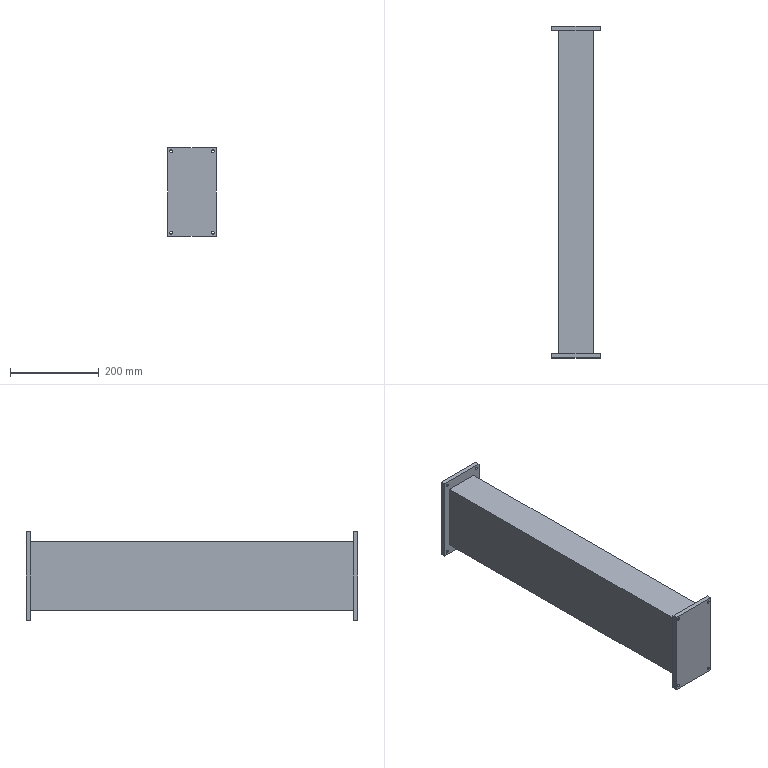Part | SolidWorks | features ICE 2, Extrusion 1 | 1 solid | 32 faces | box 110 x 750 x 200 mm | volume 9118663 mm3 | cylinder 16 | plane 16 | commonest cylinder face diameters 6.5 x16
STEP:
#1=CARTESIAN_POINT('',(-47.,750.,88.75));
#2=VERTEX_POINT('',#1);
#3=CARTESIAN_POINT('',(-47.,750.,95.25));
#4=VERTEX_POINT('',#3);
#5=CARTESIAN_POINT('',(-47.,750.,92.));
#6=DIRECTION('',(0.,1.,0.));
#7=DIRECTION('',(0.,0.,1.));
#8=AXIS2_PLACEMENT_3D('',#5,#6,#7);
#9=CIRCLE('',#8,3.25);
#10=EDGE_CURVE('',#2,#4,#9,.T.);
#11=ORIENTED_EDGE('',*,*,#10,.T.);
#12=CARTESIAN_POINT('',(-47.,740.,95.25));
#13=VERTEX_POINT('',#12);
#14=CARTESIAN_POINT('',(-47.,750.,95.25));
#15=DIRECTION('',(0.,-1.,0.));
#16=VECTOR('',#15,1000.);
#17=LINE('',#14,#16);
#18=EDGE_CURVE('',#4,#13,#17,.T.);
#19=ORIENTED_EDGE('',*,*,#18,.T.);
#20=CARTESIAN_POINT('',(-47.,740.,88.75));
#21=VERTEX_POINT('',#20);
#22=CARTESIAN_POINT('',(-47.,740.,92.));
#23=DIRECTION('',(0.,1.,0.));
#24=DIRECTION('',(0.,0.,1.));
#25=AXIS2_PLACEMENT_3D('',#22,#23,#24);
#26=CIRCLE('',#25,3.25);
#27=EDGE_CURVE('',#21,#13,#26,.T.);
#28=ORIENTED_EDGE('',*,*,#27,.F.);
#29=CARTESIAN_POINT('',(-47.,750.,88.75));
#30=DIRECTION('',(0.,-1.,0.));
#31=VECTOR('',#30,1000.);
#32=LINE('',#29,#31);
#33=EDGE_CURVE('',#2,#21,#32,.T.);
#34=ORIENTED_EDGE('',*,*,#33,.F.);
#35=EDGE_LOOP('',(#11,#19,#28,#34));
#36=FACE_OUTER_BOUND('',#35,.T.);
#37=CARTESIAN_POINT('',(-47.,750.,92.));
#38=DIRECTION('',(0.,-1.,0.));
#39=DIRECTION('',(0.,0.,-1.));
#40=AXIS2_PLACEMENT_3D('',#37,#38,#39);
#41=CYLINDRICAL_SURFACE('',#40,3.25);
#42=ADVANCED_FACE('',(#36),#41,.F.);
#43=CARTESIAN_POINT('',(47.,750.,88.75));
#44=VERTEX_POINT('',#43);
#45=CARTESIAN_POINT('',(47.,750.,95.25));
#46=VERTEX_POINT('',#45);
#47=CARTESIAN_POINT('',(47.,750.,92.));
#48=DIRECTION('',(0.,1.,0.));
#49=DIRECTION('',(0.,0.,1.));
#50=AXIS2_PLACEMENT_3D('',#47,#48,#49);
#51=CIRCLE('',#50,3.25);
#52=EDGE_CURVE('',#44,#46,#51,.T.);
#53=ORIENTED_EDGE('',*,*,#52,.T.);
#54=CARTESIAN_POINT('',(47.,740.,95.25));
#55=VERTEX_POINT('',#54);
#56=CARTESIAN_POINT('',(47.,750.,95.25));
#57=DIRECTION('',(0.,-1.,0.));
#58=VECTOR('',#57,1000.);
#59=LINE('',#56,#58);
#60=EDGE_CURVE('',#46,#55,#59,.T.);
#61=ORIENTED_EDGE('',*,*,#60,.T.);
#62=CARTESIAN_POINT('',(47.,740.,88.75));
#63=VERTEX_POINT('',#62);
#64=CARTESIAN_POINT('',(47.,740.,92.));
#65=DIRECTION('',(0.,1.,0.));
#66=DIRECTION('',(0.,0.,1.));
#67=AXIS2_PLACEMENT_3D('',#64,#65,#66);
#68=CIRCLE('',#67,3.25);
#69=EDGE_CURVE('',#63,#55,#68,.T.);
#70=ORIENTED_EDGE('',*,*,#69,.F.);
#71=CARTESIAN_POINT('',(47.,750.,88.75));
#72=DIRECTION('',(0.,-1.,0.));
#73=VECTOR('',#72,1000.);
#74=LINE('',#71,#73);
#75=EDGE_CURVE('',#44,#63,#74,.T.);
#76=ORIENTED_EDGE('',*,*,#75,.F.);
#77=EDGE_LOOP('',(#53,#61,#70,#76));
#78=FACE_OUTER_BOUND('',#77,.T.);
#79=CARTESIAN_POINT('',(47.,750.,92.));
#80=DIRECTION('',(0.,-1.,0.));
#81=DIRECTION('',(0.,0.,-1.));
#82=AXIS2_PLACEMENT_3D('',#79,#80,#81);
#83=CYLINDRICAL_SURFACE('',#82,3.25);
#84=ADVANCED_FACE('',(#78),#83,.F.);
#85=CARTESIAN_POINT('',(47.,750.,-95.25));
#86=VERTEX_POINT('',#85);
#87=CARTESIAN_POINT('',(47.,750.,-88.75));
#88=VERTEX_POINT('',#87);
#89=CARTESIAN_POINT('',(47.,750.,-92.));
#90=DIRECTION('',(0.,1.,0.));
#91=DIRECTION('',(0.,0.,1.));
#92=AXIS2_PLACEMENT_3D('',#89,#90,#91);
#93=CIRCLE('',#92,3.25);
#94=EDGE_CURVE('',#86,#88,#93,.T.);
#95=ORIENTED_EDGE('',*,*,#94,.T.);
#96=CARTESIAN_POINT('',(47.,740.,-88.75));
#97=VERTEX_POINT('',#96);
#98=CARTESIAN_POINT('',(47.,750.,-88.75));
#99=DIRECTION('',(0.,-1.,0.));
#100=VECTOR('',#99,1000.);
#101=LINE('',#98,#100);
#102=EDGE_CURVE('',#88,#97,#101,.T.);
#103=ORIENTED_EDGE('',*,*,#102,.T.);
#104=CARTESIAN_POINT('',(47.,740.,-95.25));
#105=VERTEX_POINT('',#104);
#106=CARTESIAN_POINT('',(47.,740.,-92.));
#107=DIRECTION('',(0.,1.,0.));
#108=DIRECTION('',(0.,0.,1.));
#109=AXIS2_PLACEMENT_3D('',#106,#107,#108);
#110=CIRCLE('',#109,3.25);
#111=EDGE_CURVE('',#105,#97,#110,.T.);
#112=ORIENTED_EDGE('',*,*,#111,.F.);
#113=CARTESIAN_POINT('',(47.,750.,-95.25));
#114=DIRECTION('',(0.,-1.,0.));
#115=VECTOR('',#114,1000.);
#116=LINE('',#113,#115);
#117=EDGE_CURVE('',#86,#105,#116,.T.);
#118=ORIENTED_EDGE('',*,*,#117,.F.);
#119=EDGE_LOOP('',(#95,#103,#112,#118));
#120=FACE_OUTER_BOUND('',#119,.T.);
#121=CARTESIAN_POINT('',(47.,750.,-92.));
#122=DIRECTION('',(0.,-1.,0.));
#123=DIRECTION('',(0.,0.,-1.));
#124=AXIS2_PLACEMENT_3D('',#121,#122,#123);
#125=CYLINDRICAL_SURFACE('',#124,3.25);
#126=ADVANCED_FACE('',(#120),#125,.F.);
#127=CARTESIAN_POINT('',(-47.,750.,-95.25));
#128=VERTEX_POINT('',#127);
#129=CARTESIAN_POINT('',(-47.,750.,-88.75));
#130=VERTEX_POINT('',#129);
#131=CARTESIAN_POINT('',(-47.,750.,-92.));
#132=DIRECTION('',(0.,1.,0.));
#133=DIRECTION('',(0.,0.,1.));
#134=AXIS2_PLACEMENT_3D('',#131,#132,#133);
#135=CIRCLE('',#134,3.25);
#136=EDGE_CURVE('',#128,#130,#135,.T.);
#137=ORIENTED_EDGE('',*,*,#136,.T.);
#138=CARTESIAN_POINT('',(-47.,740.,-88.75));
#139=VERTEX_POINT('',#138);
#140=CARTESIAN_POINT('',(-47.,750.,-88.75));
#141=DIRECTION('',(0.,-1.,0.));
#142=VECTOR('',#141,1000.);
#143=LINE('',#140,#142);
#144=EDGE_CURVE('',#130,#139,#143,.T.);
#145=ORIENTED_EDGE('',*,*,#144,.T.);
#146=CARTESIAN_POINT('',(-47.,740.,-95.25));
#147=VERTEX_POINT('',#146);
#148=CARTESIAN_POINT('',(-47.,740.,-92.));
#149=DIRECTION('',(0.,1.,0.));
#150=DIRECTION('',(0.,0.,1.));
#151=AXIS2_PLACEMENT_3D('',#148,#149,#150);
#152=CIRCLE('',#151,3.25);
#153=EDGE_CURVE('',#147,#139,#152,.T.);
#154=ORIENTED_EDGE('',*,*,#153,.F.);
#155=CARTESIAN_POINT('',(-47.,750.,-95.25));
#156=DIRECTION('',(0.,-1.,0.));
#157=VECTOR('',#156,1000.);
#158=LINE('',#155,#157);
#159=EDGE_CURVE('',#128,#147,#158,.T.);
#160=ORIENTED_EDGE('',*,*,#159,.F.);
#161=EDGE_LOOP('',(#137,#145,#154,#160));
#162=FACE_OUTER_BOUND('',#161,.T.);
#163=CARTESIAN_POINT('',(-47.,750.,-92.));
#164=DIRECTION('',(0.,-1.,0.));
#165=DIRECTION('',(0.,0.,-1.));
#166=AXIS2_PLACEMENT_3D('',#163,#164,#165);
#167=CYLINDRICAL_SURFACE('',#166,3.25);
#168=ADVANCED_FACE('',(#162),#167,.F.);
#169=CARTESIAN_POINT('',(-47.,10.,88.75));
#170=VERTEX_POINT('',#169);
#171=CARTESIAN_POINT('',(-47.,10.,95.25));
#172=VERTEX_POINT('',#171);
#173=CARTESIAN_POINT('',(-47.,10.,92.));
#174=DIRECTION('',(0.,1.,0.));
#175=DIRECTION('',(0.,0.,1.));
#176=AXIS2_PLACEMENT_3D('',#173,#174,#175);
#177=CIRCLE('',#176,3.25);
#178=EDGE_CURVE('',#170,#172,#177,.T.);
#179=ORIENTED_EDGE('',*,*,#178,.T.);
#180=CARTESIAN_POINT('',(-47.,0.,95.25));
#181=VERTEX_POINT('',#180);
#182=CARTESIAN_POINT('',(-47.,10.,95.25));
#183=DIRECTION('',(0.,-1.,0.));
#184=VECTOR('',#183,1000.);
#185=LINE('',#182,#184);
#186=EDGE_CURVE('',#172,#181,#185,.T.);
#187=ORIENTED_EDGE('',*,*,#186,.T.);
#188=CARTESIAN_POINT('',(-47.,0.,88.75));
#189=VERTEX_POINT('',#188);
#190=CARTESIAN_POINT('',(-47.,0.,92.));
#191=DIRECTION('',(0.,1.,0.));
#192=DIRECTION('',(0.,0.,1.));
#193=AXIS2_PLACEMENT_3D('',#190,#191,#192);
#194=CIRCLE('',#193,3.25);
#195=EDGE_CURVE('',#189,#181,#194,.T.);
#196=ORIENTED_EDGE('',*,*,#195,.F.);
#197=CARTESIAN_POINT('',(-47.,10.,88.75));
#198=DIRECTION('',(0.,-1.,0.));
#199=VECTOR('',#198,1000.);
#200=LINE('',#197,#199);
#201=EDGE_CURVE('',#170,#189,#200,.T.);
#202=ORIENTED_EDGE('',*,*,#201,.F.);
#203=EDGE_LOOP('',(#179,#187,#196,#202));
#204=FACE_OUTER_BOUND('',#203,.T.);
#205=CARTESIAN_POINT('',(-47.,10.,92.));
#206=DIRECTION('',(0.,-1.,0.));
#207=DIRECTION('',(0.,0.,-1.));
#208=AXIS2_PLACEMENT_3D('',#205,#206,#207);
#209=CYLINDRICAL_SURFACE('',#208,3.25);
#210=ADVANCED_FACE('',(#204),#209,.F.);
#211=CARTESIAN_POINT('',(47.,10.,88.75));
#212=VERTEX_POINT('',#211);
#213=CARTESIAN_POINT('',(47.,10.,95.25));
#214=VERTEX_POINT('',#213);
#215=CARTESIAN_POINT('',(47.,10.,92.));
#216=DIRECTION('',(0.,1.,0.));
#217=DIRECTION('',(0.,0.,1.));
#218=AXIS2_PLACEMENT_3D('',#215,#216,#217);
#219=CIRCLE('',#218,3.25);
#220=EDGE_CURVE('',#212,#214,#219,.T.);
#221=ORIENTED_EDGE('',*,*,#220,.T.);
#222=CARTESIAN_POINT('',(47.,0.,95.25));
#223=VERTEX_POINT('',#222);
#224=CARTESIAN_POINT('',(47.,10.,95.25));
#225=DIRECTION('',(0.,-1.,0.));
#226=VECTOR('',#225,1000.);
#227=LINE('',#224,#226);
#228=EDGE_CURVE('',#214,#223,#227,.T.);
#229=ORIENTED_EDGE('',*,*,#228,.T.);
#230=CARTESIAN_POINT('',(47.,0.,88.75));
#231=VERTEX_POINT('',#230);
#232=CARTESIAN_POINT('',(47.,0.,92.));
#233=DIRECTION('',(0.,1.,0.));
#234=DIRECTION('',(0.,0.,1.));
#235=AXIS2_PLACEMENT_3D('',#232,#233,#234);
#236=CIRCLE('',#235,3.25);
#237=EDGE_CURVE('',#231,#223,#236,.T.);
#238=ORIENTED_EDGE('',*,*,#237,.F.);
#239=CARTESIAN_POINT('',(47.,10.,88.75));
#240=DIRECTION('',(0.,-1.,0.));
#241=VECTOR('',#240,1000.);
#242=LINE('',#239,#241);
#243=EDGE_CURVE('',#212,#231,#242,.T.);
#244=ORIENTED_EDGE('',*,*,#243,.F.);
#245=EDGE_LOOP('',(#221,#229,#238,#244));
#246=FACE_OUTER_BOUND('',#245,.T.);
#247=CARTESIAN_POINT('',(47.,10.,92.));
#248=DIRECTION('',(0.,-1.,0.));
#249=DIRECTION('',(0.,0.,-1.));
#250=AXIS2_PLACEMENT_3D('',#247,#248,#249);
#251=CYLINDRICAL_SURFACE('',#250,3.25);
#252=ADVANCED_FACE('',(#246),#251,.F.);
#253=CARTESIAN_POINT('',(47.,10.,-95.25));
#254=VERTEX_POINT('',#253);
#255=CARTESIAN_POINT('',(47.,10.,-88.75));
#256=VERTEX_POINT('',#255);
#257=CARTESIAN_POINT('',(47.,10.,-92.));
#258=DIRECTION('',(0.,1.,0.));
#259=DIRECTION('',(0.,0.,1.));
#260=AXIS2_PLACEMENT_3D('',#257,#258,#259);
#261=CIRCLE('',#260,3.25);
#262=EDGE_CURVE('',#254,#256,#261,.T.);
#263=ORIENTED_EDGE('',*,*,#262,.T.);
#264=CARTESIAN_POINT('',(47.,0.,-88.75));
#265=VERTEX_POINT('',#264);
#266=CARTESIAN_POINT('',(47.,10.,-88.75));
#267=DIRECTION('',(0.,-1.,0.));
#268=VECTOR('',#267,1000.);
#269=LINE('',#266,#268);
#270=EDGE_CURVE('',#256,#265,#269,.T.);
#271=ORIENTED_EDGE('',*,*,#270,.T.);
#272=CARTESIAN_POINT('',(47.,0.,-95.25));
#273=VERTEX_POINT('',#272);
#274=CARTESIAN_POINT('',(47.,0.,-92.));
#275=DIRECTION('',(0.,1.,0.));
#276=DIRECTION('',(0.,0.,1.));
#277=AXIS2_PLACEMENT_3D('',#274,#275,#276);
#278=CIRCLE('',#277,3.25);
#279=EDGE_CURVE('',#273,#265,#278,.T.);
#280=ORIENTED_EDGE('',*,*,#279,.F.);
#281=CARTESIAN_POINT('',(47.,10.,-95.25));
#282=DIRECTION('',(0.,-1.,0.));
#283=VECTOR('',#282,1000.);
#284=LINE('',#281,#283);
#285=EDGE_CURVE('',#254,#273,#284,.T.);
#286=ORIENTED_EDGE('',*,*,#285,.F.);
#287=EDGE_LOOP('',(#263,#271,#280,#286));
#288=FACE_OUTER_BOUND('',#287,.T.);
#289=CARTESIAN_POINT('',(47.,10.,-92.));
#290=DIRECTION('',(0.,-1.,0.));
#291=DIRECTION('',(0.,0.,-1.));
#292=AXIS2_PLACEMENT_3D('',#289,#290,#291);
#293=CYLINDRICAL_SURFACE('',#292,3.25);
#294=ADVANCED_FACE('',(#288),#293,.F.);
#295=CARTESIAN_POINT('',(-47.,10.,-95.25));
#296=VERTEX_POINT('',#295);
#297=CARTESIAN_POINT('',(-47.,10.,-88.75));
#298=VERTEX_POINT('',#297);
#299=CARTESIAN_POINT('',(-47.,10.,-92.));
#300=DIRECTION('',(0.,1.,0.));
#301=DIRECTION('',(0.,0.,1.));
#302=AXIS2_PLACEMENT_3D('',#299,#300,#301);
#303=CIRCLE('',#302,3.25);
#304=EDGE_CURVE('',#296,#298,#303,.T.);
#305=ORIENTED_EDGE('',*,*,#304,.T.);
#306=CARTESIAN_POINT('',(-47.,0.,-88.75));
#307=VERTEX_POINT('',#306);
#308=CARTESIAN_POINT('',(-47.,10.,-88.75));
#309=DIRECTION('',(0.,-1.,0.));
#310=VECTOR('',#309,1000.);
#311=LINE('',#308,#310);
#312=EDGE_CURVE('',#298,#307,#311,.T.);
#313=ORIENTED_EDGE('',*,*,#312,.T.);
#314=CARTESIAN_POINT('',(-47.,0.,-95.25));
#315=VERTEX_POINT('',#314);
#316=CARTESIAN_POINT('',(-47.,0.,-92.));
#317=DIRECTION('',(0.,1.,0.));
#318=DIRECTION('',(0.,0.,1.));
#319=AXIS2_PLACEMENT_3D('',#316,#317,#318);
#320=CIRCLE('',#319,3.25);
#321=EDGE_CURVE('',#315,#307,#320,.T.);
#322=ORIENTED_EDGE('',*,*,#321,.F.);
#323=CARTESIAN_POINT('',(-47.,10.,-95.25));
#324=DIRECTION('',(0.,-1.,0.));
#325=VECTOR('',#324,1000.);
#326=LINE('',#323,#325);
#327=EDGE_CURVE('',#296,#315,#326,.T.);
#328=ORIENTED_EDGE('',*,*,#327,.F.);
#329=EDGE_LOOP('',(#305,#313,#322,#328));
#330=FACE_OUTER_BOUND('',#329,.T.);
#331=CARTESIAN_POINT('',(-47.,10.,-92.));
#332=DIRECTION('',(0.,-1.,0.));
#333=DIRECTION('',(0.,0.,-1.));
#334=AXIS2_PLACEMENT_3D('',#331,#332,#333);
#335=CYLINDRICAL_SURFACE('',#334,3.25);
#336=ADVANCED_FACE('',(#330),#335,.F.);
#337=ORIENTED_EDGE('',*,*,#178,.F.);
#338=CARTESIAN_POINT('',(-47.,10.,92.));
#339=DIRECTION('',(0.,1.,0.));
#340=DIRECTION('',(0.,0.,1.));
#341=AXIS2_PLACEMENT_3D('',#338,#339,#340);
#342=CIRCLE('',#341,3.25);
#343=EDGE_CURVE('',#172,#170,#342,.T.);
#344=ORIENTED_EDGE('',*,*,#343,.F.);
#345=EDGE_LOOP('',(#337,#344));
#346=FACE_BOUND('',#345,.T.);
#347=ORIENTED_EDGE('',*,*,#220,.F.);
#348=CARTESIAN_POINT('',(47.,10.,92.));
#349=DIRECTION('',(0.,1.,0.));
#350=DIRECTION('',(0.,0.,1.));
#351=AXIS2_PLACEMENT_3D('',#348,#349,#350);
#352=CIRCLE('',#351,3.25);
#353=EDGE_CURVE('',#214,#212,#352,.T.);
#354=ORIENTED_EDGE('',*,*,#353,.F.);
#355=EDGE_LOOP('',(#347,#354));
#356=FACE_BOUND('',#355,.T.);
#357=ORIENTED_EDGE('',*,*,#262,.F.);
#358=CARTESIAN_POINT('',(47.,10.,-92.));
#359=DIRECTION('',(0.,1.,0.));
#360=DIRECTION('',(0.,0.,1.));
#361=AXIS2_PLACEMENT_3D('',#358,#359,#360);
#362=CIRCLE('',#361,3.25);
#363=EDGE_CURVE('',#256,#254,#362,.T.);
#364=ORIENTED_EDGE('',*,*,#363,.F.);
#365=EDGE_LOOP('',(#357,#364));
#366=FACE_BOUND('',#365,.T.);
#367=ORIENTED_EDGE('',*,*,#304,.F.);
#368=CARTESIAN_POINT('',(-47.,10.,-92.));
#369=DIRECTION('',(0.,1.,0.));
#370=DIRECTION('',(0.,0.,1.));
#371=AXIS2_PLACEMENT_3D('',#368,#369,#370);
#372=CIRCLE('',#371,3.25);
#373=EDGE_CURVE('',#298,#296,#372,.T.);
#374=ORIENTED_EDGE('',*,*,#373,.F.);
#375=EDGE_LOOP('',(#367,#374));
#376=FACE_BOUND('',#375,.T.);
#377=CARTESIAN_POINT('',(55.,10.,100.));
#378=VERTEX_POINT('',#377);
#379=CARTESIAN_POINT('',(55.,10.,-100.));
#380=VERTEX_POINT('',#379);
#381=CARTESIAN_POINT('',(55.,10.,100.));
#382=DIRECTION('',(0.,0.,-1.));
#383=VECTOR('',#382,1000.);
#384=LINE('',#381,#383);
#385=EDGE_CURVE('',#378,#380,#384,.T.);
#386=ORIENTED_EDGE('',*,*,#385,.T.);
#387=CARTESIAN_POINT('',(-55.,10.,-100.));
#388=VERTEX_POINT('',#387);
#389=CARTESIAN_POINT('',(-55.,10.,-100.));
#390=DIRECTION('',(-1.,0.,0.));
#391=VECTOR('',#390,1000.);
#392=LINE('',#389,#391);
#393=EDGE_CURVE('',#380,#388,#392,.T.);
#394=ORIENTED_EDGE('',*,*,#393,.T.);
#395=CARTESIAN_POINT('',(-55.,10.,100.));
#396=VERTEX_POINT('',#395);
#397=CARTESIAN_POINT('',(-55.,10.,100.));
#398=DIRECTION('',(0.,0.,1.));
#399=VECTOR('',#398,1000.);
#400=LINE('',#397,#399);
#401=EDGE_CURVE('',#388,#396,#400,.T.);
#402=ORIENTED_EDGE('',*,*,#401,.T.);
#403=CARTESIAN_POINT('',(-55.,10.,100.));
#404=DIRECTION('',(1.,0.,0.));
#405=VECTOR('',#404,1000.);
#406=LINE('',#403,#405);
#407=EDGE_CURVE('',#396,#378,#406,.T.);
#408=ORIENTED_EDGE('',*,*,#407,.T.);
#409=EDGE_LOOP('',(#386,#394,#402,#408));
#410=FACE_OUTER_BOUND('',#409,.T.);
#411=CARTESIAN_POINT('',(38.672,10.,76.878));
#412=VERTEX_POINT('',#411);
#413=CARTESIAN_POINT('',(38.672,10.,-76.878));
#414=VERTEX_POINT('',#413);
#415=CARTESIAN_POINT('',(38.672,10.,76.878));
#416=DIRECTION('',(0.,0.,-1.));
#417=VECTOR('',#416,1000.);
#418=LINE('',#415,#417);
#419=EDGE_CURVE('',#412,#414,#418,.T.);
#420=ORIENTED_EDGE('',*,*,#419,.F.);
#421=CARTESIAN_POINT('',(-38.672,10.,76.878));
#422=VERTEX_POINT('',#421);
#423=CARTESIAN_POINT('',(-38.672,10.,76.878));
#424=DIRECTION('',(1.,0.,0.));
#425=VECTOR('',#424,1000.);
#426=LINE('',#423,#425);
#427=EDGE_CURVE('',#422,#412,#426,.T.);
#428=ORIENTED_EDGE('',*,*,#427,.F.);
#429=CARTESIAN_POINT('',(-38.672,10.,-76.878));
#430=VERTEX_POINT('',#429);
#431=CARTESIAN_POINT('',(-38.672,10.,76.878));
#432=DIRECTION('',(0.,0.,1.));
#433=VECTOR('',#432,1000.);
#434=LINE('',#431,#433);
#435=EDGE_CURVE('',#430,#422,#434,.T.);
#436=ORIENTED_EDGE('',*,*,#435,.F.);
#437=CARTESIAN_POINT('',(-38.672,10.,-76.878));
#438=DIRECTION('',(-1.,0.,0.));
#439=VECTOR('',#438,1000.);
#440=LINE('',#437,#439);
#441=EDGE_CURVE('',#414,#430,#440,.T.);
#442=ORIENTED_EDGE('',*,*,#441,.F.);
#443=EDGE_LOOP('',(#420,#428,#436,#442));
#444=FACE_BOUND('',#443,.T.);
#445=CARTESIAN_POINT('',(0.,10.,0.));
#446=DIRECTION('',(0.,-1.,0.));
#447=DIRECTION('',(0.,0.,-1.));
#448=AXIS2_PLACEMENT_3D('',#445,#446,#447);
#449=PLANE('',#448);
#450=ADVANCED_FACE('',(#346,#356,#366,#376,#410,#444),#449,.F.);
#451=ORIENTED_EDGE('',*,*,#237,.T.);
#452=CARTESIAN_POINT('',(47.,0.,92.));
#453=DIRECTION('',(0.,1.,0.));
#454=DIRECTION('',(0.,0.,1.));
#455=AXIS2_PLACEMENT_3D('',#452,#453,#454);
#456=CIRCLE('',#455,3.25);
#457=EDGE_CURVE('',#223,#231,#456,.T.);
#458=ORIENTED_EDGE('',*,*,#457,.T.);
#459=EDGE_LOOP('',(#451,#458));
#460=FACE_BOUND('',#459,.T.);
#461=ORIENTED_EDGE('',*,*,#321,.T.);
#462=CARTESIAN_POINT('',(-47.,0.,-92.));
#463=DIRECTION('',(0.,1.,0.));
#464=DIRECTION('',(0.,0.,1.));
#465=AXIS2_PLACEMENT_3D('',#462,#463,#464);
#466=CIRCLE('',#465,3.25);
#467=EDGE_CURVE('',#307,#315,#466,.T.);
#468=ORIENTED_EDGE('',*,*,#467,.T.);
#469=EDGE_LOOP('',(#461,#468));
#470=FACE_BOUND('',#469,.T.);
#471=CARTESIAN_POINT('',(55.,0.,100.));
#472=VERTEX_POINT('',#471);
#473=CARTESIAN_POINT('',(55.,0.,-100.));
#474=VERTEX_POINT('',#473);
#475=CARTESIAN_POINT('',(55.,0.,100.));
#476=DIRECTION('',(0.,0.,-1.));
#477=VECTOR('',#476,1000.);
#478=LINE('',#475,#477);
#479=EDGE_CURVE('',#472,#474,#478,.T.);
#480=ORIENTED_EDGE('',*,*,#479,.F.);
#481=CARTESIAN_POINT('',(-55.,0.,100.));
#482=VERTEX_POINT('',#481);
#483=CARTESIAN_POINT('',(-55.,0.,100.));
#484=DIRECTION('',(1.,0.,0.));
#485=VECTOR('',#484,1000.);
#486=LINE('',#483,#485);
#487=EDGE_CURVE('',#482,#472,#486,.T.);
#488=ORIENTED_EDGE('',*,*,#487,.F.);
#489=CARTESIAN_POINT('',(-55.,0.,-100.));
#490=VERTEX_POINT('',#489);
#491=CARTESIAN_POINT('',(-55.,0.,100.));
#492=DIRECTION('',(0.,0.,1.));
#493=VECTOR('',#492,1000.);
#494=LINE('',#491,#493);
#495=EDGE_CURVE('',#490,#482,#494,.T.);
#496=ORIENTED_EDGE('',*,*,#495,.F.);
#497=CARTESIAN_POINT('',(-55.,0.,-100.));
#498=DIRECTION('',(-1.,0.,0.));
#499=VECTOR('',#498,1000.);
#500=LINE('',#497,#499);
#501=EDGE_CURVE('',#474,#490,#500,.T.);
#502=ORIENTED_EDGE('',*,*,#501,.F.);
#503=EDGE_LOOP('',(#480,#488,#496,#502));
#504=FACE_OUTER_BOUND('',#503,.T.);
#505=ORIENTED_EDGE('',*,*,#279,.T.);
#506=CARTESIAN_POINT('',(47.,0.,-92.));
#507=DIRECTION('',(0.,1.,0.));
#508=DIRECTION('',(0.,0.,1.));
#509=AXIS2_PLACEMENT_3D('',#506,#507,#508);
#510=CIRCLE('',#509,3.25);
#511=EDGE_CURVE('',#265,#273,#510,.T.);
#512=ORIENTED_EDGE('',*,*,#511,.T.);
#513=EDGE_LOOP('',(#505,#512));
#514=FACE_BOUND('',#513,.T.);
#515=ORIENTED_EDGE('',*,*,#195,.T.);
#516=CARTESIAN_POINT('',(-47.,0.,92.));
#517=DIRECTION('',(0.,1.,0.));
#518=DIRECTION('',(0.,0.,1.));
#519=AXIS2_PLACEMENT_3D('',#516,#517,#518);
#520=CIRCLE('',#519,3.25);
#521=EDGE_CURVE('',#181,#189,#520,.T.);
#522=ORIENTED_EDGE('',*,*,#521,.T.);
#523=EDGE_LOOP('',(#515,#522));
#524=FACE_BOUND('',#523,.T.);
#525=CARTESIAN_POINT('',(0.,0.,0.));
#526=DIRECTION('',(0.,-1.,0.));
#527=DIRECTION('',(0.,0.,-1.));
#528=AXIS2_PLACEMENT_3D('',#525,#526,#527);
#529=PLANE('',#528);
#530=ADVANCED_FACE('',(#460,#470,#504,#514,#524),#529,.T.);
#531=ORIENTED_EDGE('',*,*,#479,.T.);
#532=CARTESIAN_POINT('',(55.,10.,-100.));
#533=DIRECTION('',(0.,-1.,0.));
#534=VECTOR('',#533,1000.);
#535=LINE('',#532,#534);
#536=EDGE_CURVE('',#380,#474,#535,.T.);
#537=ORIENTED_EDGE('',*,*,#536,.F.);
#538=ORIENTED_EDGE('',*,*,#385,.F.);
#539=CARTESIAN_POINT('',(55.,10.,100.));
#540=DIRECTION('',(0.,-1.,0.));
#541=VECTOR('',#540,1000.);
#542=LINE('',#539,#541);
#543=EDGE_CURVE('',#378,#472,#542,.T.);
#544=ORIENTED_EDGE('',*,*,#543,.T.);
#545=EDGE_LOOP('',(#531,#537,#538,#544));
#546=FACE_OUTER_BOUND('',#545,.T.);
#547=CARTESIAN_POINT('',(55.,10.,100.));
#548=DIRECTION('',(-1.,0.,0.));
#549=DIRECTION('',(0.,0.,1.));
#550=AXIS2_PLACEMENT_3D('',#547,#548,#549);
#551=PLANE('',#550);
#552=ADVANCED_FACE('',(#546),#551,.F.);
#553=ORIENTED_EDGE('',*,*,#501,.T.);
#554=CARTESIAN_POINT('',(-55.,10.,-100.));
#555=DIRECTION('',(0.,-1.,0.));
#556=VECTOR('',#555,1000.);
#557=LINE('',#554,#556);
#558=EDGE_CURVE('',#388,#490,#557,.T.);
#559=ORIENTED_EDGE('',*,*,#558,.F.);
#560=ORIENTED_EDGE('',*,*,#393,.F.);
#561=ORIENTED_EDGE('',*,*,#536,.T.);
#562=EDGE_LOOP('',(#553,#559,#560,#561));
#563=FACE_OUTER_BOUND('',#562,.T.);
#564=CARTESIAN_POINT('',(-55.,10.,-100.));
#565=DIRECTION('',(0.,0.,1.));
#566=DIRECTION('',(1.,0.,0.));
#567=AXIS2_PLACEMENT_3D('',#564,#565,#566);
#568=PLANE('',#567);
#569=ADVANCED_FACE('',(#563),#568,.F.);
#570=ORIENTED_EDGE('',*,*,#495,.T.);
#571=CARTESIAN_POINT('',(-55.,10.,100.));
#572=DIRECTION('',(0.,-1.,0.));
#573=VECTOR('',#572,1000.);
#574=LINE('',#571,#573);
#575=EDGE_CURVE('',#396,#482,#574,.T.);
#576=ORIENTED_EDGE('',*,*,#575,.F.);
#577=ORIENTED_EDGE('',*,*,#401,.F.);
#578=ORIENTED_EDGE('',*,*,#558,.T.);
#579=EDGE_LOOP('',(#570,#576,#577,#578));
#580=FACE_OUTER_BOUND('',#579,.T.);
#581=CARTESIAN_POINT('',(-55.,10.,100.));
#582=DIRECTION('',(1.,0.,0.));
#583=DIRECTION('',(0.,0.,-1.));
#584=AXIS2_PLACEMENT_3D('',#581,#582,#583);
#585=PLANE('',#584);
#586=ADVANCED_FACE('',(#580),#585,.F.);
#587=ORIENTED_EDGE('',*,*,#487,.T.);
#588=ORIENTED_EDGE('',*,*,#543,.F.);
#589=ORIENTED_EDGE('',*,*,#407,.F.);
#590=ORIENTED_EDGE('',*,*,#575,.T.);
#591=EDGE_LOOP('',(#587,#588,#589,#590));
#592=FACE_OUTER_BOUND('',#591,.T.);
#593=CARTESIAN_POINT('',(-55.,10.,100.));
#594=DIRECTION('',(0.,0.,-1.));
#595=DIRECTION('',(-1.,0.,0.));
#596=AXIS2_PLACEMENT_3D('',#593,#594,#595);
#597=PLANE('',#596);
#598=ADVANCED_FACE('',(#592),#597,.F.);
#599=ORIENTED_EDGE('',*,*,#312,.F.);
#600=ORIENTED_EDGE('',*,*,#373,.T.);
#601=ORIENTED_EDGE('',*,*,#327,.T.);
#602=ORIENTED_EDGE('',*,*,#467,.F.);
#603=EDGE_LOOP('',(#599,#600,#601,#602));
#604=FACE_OUTER_BOUND('',#603,.T.);
#605=CARTESIAN_POINT('',(-47.,10.,-92.));
#606=DIRECTION('',(0.,-1.,0.));
#607=DIRECTION('',(0.,0.,-1.));
#608=AXIS2_PLACEMENT_3D('',#605,#606,#607);
#609=CYLINDRICAL_SURFACE('',#608,3.25);
#610=ADVANCED_FACE('',(#604),#609,.F.);
#611=ORIENTED_EDGE('',*,*,#270,.F.);
#612=ORIENTED_EDGE('',*,*,#363,.T.);
#613=ORIENTED_EDGE('',*,*,#285,.T.);
#614=ORIENTED_EDGE('',*,*,#511,.F.);
#615=EDGE_LOOP('',(#611,#612,#613,#614));
#616=FACE_OUTER_BOUND('',#615,.T.);
#617=CARTESIAN_POINT('',(47.,10.,-92.));
#618=DIRECTION('',(0.,-1.,0.));
#619=DIRECTION('',(0.,0.,-1.));
#620=AXIS2_PLACEMENT_3D('',#617,#618,#619);
#621=CYLINDRICAL_SURFACE('',#620,3.25);
#622=ADVANCED_FACE('',(#616),#621,.F.);
#623=ORIENTED_EDGE('',*,*,#228,.F.);
#624=ORIENTED_EDGE('',*,*,#353,.T.);
#625=ORIENTED_EDGE('',*,*,#243,.T.);
#626=ORIENTED_EDGE('',*,*,#457,.F.);
#627=EDGE_LOOP('',(#623,#624,#625,#626));
#628=FACE_OUTER_BOUND('',#627,.T.);
#629=CARTESIAN_POINT('',(47.,10.,92.));
#630=DIRECTION('',(0.,-1.,0.));
#631=DIRECTION('',(0.,0.,-1.));
#632=AXIS2_PLACEMENT_3D('',#629,#630,#631);
#633=CYLINDRICAL_SURFACE('',#632,3.25);
#634=ADVANCED_FACE('',(#628),#633,.F.);
#635=ORIENTED_EDGE('',*,*,#186,.F.);
#636=ORIENTED_EDGE('',*,*,#343,.T.);
#637=ORIENTED_EDGE('',*,*,#201,.T.);
#638=ORIENTED_EDGE('',*,*,#521,.F.);
#639=EDGE_LOOP('',(#635,#636,#637,#638));
#640=FACE_OUTER_BOUND('',#639,.T.);
#641=CARTESIAN_POINT('',(-47.,10.,92.));
#642=DIRECTION('',(0.,-1.,0.));
#643=DIRECTION('',(0.,0.,-1.));
#644=AXIS2_PLACEMENT_3D('',#641,#642,#643);
#645=CYLINDRICAL_SURFACE('',#644,3.25);
#646=ADVANCED_FACE('',(#640),#645,.F.);
#647=ORIENTED_EDGE('',*,*,#419,.T.);
#648=CARTESIAN_POINT('',(38.672,740.,-76.878));
#649=VERTEX_POINT('',#648);
#650=CARTESIAN_POINT('',(38.672,740.,-76.878));
#651=DIRECTION('',(0.,-1.,0.));
#652=VECTOR('',#651,1000.);
#653=LINE('',#650,#652);
#654=EDGE_CURVE('',#649,#414,#653,.T.);
#655=ORIENTED_EDGE('',*,*,#654,.F.);
#656=CARTESIAN_POINT('',(38.672,740.,76.878));
#657=VERTEX_POINT('',#656);
#658=CARTESIAN_POINT('',(38.672,740.,76.878));
#659=DIRECTION('',(0.,0.,-1.));
#660=VECTOR('',#659,1000.);
#661=LINE('',#658,#660);
#662=EDGE_CURVE('',#657,#649,#661,.T.);
#663=ORIENTED_EDGE('',*,*,#662,.F.);
#664=CARTESIAN_POINT('',(38.672,740.,76.878));
#665=DIRECTION('',(0.,-1.,0.));
#666=VECTOR('',#665,1000.);
#667=LINE('',#664,#666);
#668=EDGE_CURVE('',#657,#412,#667,.T.);
#669=ORIENTED_EDGE('',*,*,#668,.T.);
#670=EDGE_LOOP('',(#647,#655,#663,#669));
#671=FACE_OUTER_BOUND('',#670,.T.);
#672=CARTESIAN_POINT('',(38.672,740.,76.878));
#673=DIRECTION('',(-1.,0.,0.));
#674=DIRECTION('',(0.,0.,1.));
#675=AXIS2_PLACEMENT_3D('',#672,#673,#674);
#676=PLANE('',#675);
#677=ADVANCED_FACE('',(#671),#676,.F.);
#678=ORIENTED_EDGE('',*,*,#441,.T.);
#679=CARTESIAN_POINT('',(-38.672,740.,-76.878));
#680=VERTEX_POINT('',#679);
#681=CARTESIAN_POINT('',(-38.672,740.,-76.878));
#682=DIRECTION('',(0.,-1.,0.));
#683=VECTOR('',#682,1000.);
#684=LINE('',#681,#683);
#685=EDGE_CURVE('',#680,#430,#684,.T.);
#686=ORIENTED_EDGE('',*,*,#685,.F.);
#687=CARTESIAN_POINT('',(-38.672,740.,-76.878));
#688=DIRECTION('',(-1.,0.,0.));
#689=VECTOR('',#688,1000.);
#690=LINE('',#687,#689);
#691=EDGE_CURVE('',#649,#680,#690,.T.);
#692=ORIENTED_EDGE('',*,*,#691,.F.);
#693=ORIENTED_EDGE('',*,*,#654,.T.);
#694=EDGE_LOOP('',(#678,#686,#692,#693));
#695=FACE_OUTER_BOUND('',#694,.T.);
#696=CARTESIAN_POINT('',(-38.672,740.,-76.878));
#697=DIRECTION('',(0.,0.,1.));
#698=DIRECTION('',(1.,0.,0.));
#699=AXIS2_PLACEMENT_3D('',#696,#697,#698);
#700=PLANE('',#699);
#701=ADVANCED_FACE('',(#695),#700,.F.);
#702=ORIENTED_EDGE('',*,*,#435,.T.);
#703=CARTESIAN_POINT('',(-38.672,740.,76.878));
#704=VERTEX_POINT('',#703);
#705=CARTESIAN_POINT('',(-38.672,740.,76.878));
#706=DIRECTION('',(0.,-1.,0.));
#707=VECTOR('',#706,1000.);
#708=LINE('',#705,#707);
#709=EDGE_CURVE('',#704,#422,#708,.T.);
#710=ORIENTED_EDGE('',*,*,#709,.F.);
#711=CARTESIAN_POINT('',(-38.672,740.,76.878));
#712=DIRECTION('',(0.,0.,1.));
#713=VECTOR('',#712,1000.);
#714=LINE('',#711,#713);
#715=EDGE_CURVE('',#680,#704,#714,.T.);
#716=ORIENTED_EDGE('',*,*,#715,.F.);
#717=ORIENTED_EDGE('',*,*,#685,.T.);
#718=EDGE_LOOP('',(#702,#710,#716,#717));
#719=FACE_OUTER_BOUND('',#718,.T.);
#720=CARTESIAN_POINT('',(-38.672,740.,76.878));
#721=DIRECTION('',(1.,0.,0.));
#722=DIRECTION('',(0.,0.,-1.));
#723=AXIS2_PLACEMENT_3D('',#720,#721,#722);
#724=PLANE('',#723);
#725=ADVANCED_FACE('',(#719),#724,.F.);
#726=ORIENTED_EDGE('',*,*,#427,.T.);
#727=ORIENTED_EDGE('',*,*,#668,.F.);
#728=CARTESIAN_POINT('',(-38.672,740.,76.878));
#729=DIRECTION('',(1.,0.,0.));
#730=VECTOR('',#729,1000.);
#731=LINE('',#728,#730);
#732=EDGE_CURVE('',#704,#657,#731,.T.);
#733=ORIENTED_EDGE('',*,*,#732,.F.);
#734=ORIENTED_EDGE('',*,*,#709,.T.);
#735=EDGE_LOOP('',(#726,#727,#733,#734));
#736=FACE_OUTER_BOUND('',#735,.T.);
#737=CARTESIAN_POINT('',(-38.672,740.,76.878));
#738=DIRECTION('',(0.,0.,-1.));
#739=DIRECTION('',(-1.,0.,0.));
#740=AXIS2_PLACEMENT_3D('',#737,#738,#739);
#741=PLANE('',#740);
#742=ADVANCED_FACE('',(#736),#741,.F.);
#743=CARTESIAN_POINT('',(55.,750.,100.));
#744=VERTEX_POINT('',#743);
#745=CARTESIAN_POINT('',(55.,750.,-100.));
#746=VERTEX_POINT('',#745);
#747=CARTESIAN_POINT('',(55.,750.,100.));
#748=DIRECTION('',(0.,0.,-1.));
#749=VECTOR('',#748,1000.);
#750=LINE('',#747,#749);
#751=EDGE_CURVE('',#744,#746,#750,.T.);
#752=ORIENTED_EDGE('',*,*,#751,.T.);
#753=CARTESIAN_POINT('',(-55.,750.,-100.));
#754=VERTEX_POINT('',#753);
#755=CARTESIAN_POINT('',(-55.,750.,-100.));
#756=DIRECTION('',(-1.,0.,0.));
#757=VECTOR('',#756,1000.);
#758=LINE('',#755,#757);
#759=EDGE_CURVE('',#746,#754,#758,.T.);
#760=ORIENTED_EDGE('',*,*,#759,.T.);
#761=CARTESIAN_POINT('',(-55.,750.,100.));
#762=VERTEX_POINT('',#761);
#763=CARTESIAN_POINT('',(-55.,750.,100.));
#764=DIRECTION('',(0.,0.,1.));
#765=VECTOR('',#764,1000.);
#766=LINE('',#763,#765);
#767=EDGE_CURVE('',#754,#762,#766,.T.);
#768=ORIENTED_EDGE('',*,*,#767,.T.);
#769=CARTESIAN_POINT('',(-55.,750.,100.));
#770=DIRECTION('',(1.,0.,0.));
#771=VECTOR('',#770,1000.);
#772=LINE('',#769,#771);
#773=EDGE_CURVE('',#762,#744,#772,.T.);
#774=ORIENTED_EDGE('',*,*,#773,.T.);
#775=EDGE_LOOP('',(#752,#760,#768,#774));
#776=FACE_OUTER_BOUND('',#775,.T.);
#777=ORIENTED_EDGE('',*,*,#136,.F.);
#778=CARTESIAN_POINT('',(-47.,750.,-92.));
#779=DIRECTION('',(0.,1.,0.));
#780=DIRECTION('',(0.,0.,1.));
#781=AXIS2_PLACEMENT_3D('',#778,#779,#780);
#782=CIRCLE('',#781,3.25);
#783=EDGE_CURVE('',#130,#128,#782,.T.);
#784=ORIENTED_EDGE('',*,*,#783,.F.);
#785=EDGE_LOOP('',(#777,#784));
#786=FACE_BOUND('',#785,.T.);
#787=ORIENTED_EDGE('',*,*,#94,.F.);
#788=CARTESIAN_POINT('',(47.,750.,-92.));
#789=DIRECTION('',(0.,1.,0.));
#790=DIRECTION('',(0.,0.,1.));
#791=AXIS2_PLACEMENT_3D('',#788,#789,#790);
#792=CIRCLE('',#791,3.25);
#793=EDGE_CURVE('',#88,#86,#792,.T.);
#794=ORIENTED_EDGE('',*,*,#793,.F.);
#795=EDGE_LOOP('',(#787,#794));
#796=FACE_BOUND('',#795,.T.);
#797=ORIENTED_EDGE('',*,*,#52,.F.);
#798=CARTESIAN_POINT('',(47.,750.,92.));
#799=DIRECTION('',(0.,1.,0.));
#800=DIRECTION('',(0.,0.,1.));
#801=AXIS2_PLACEMENT_3D('',#798,#799,#800);
#802=CIRCLE('',#801,3.25);
#803=EDGE_CURVE('',#46,#44,#802,.T.);
#804=ORIENTED_EDGE('',*,*,#803,.F.);
#805=EDGE_LOOP('',(#797,#804));
#806=FACE_BOUND('',#805,.T.);
#807=ORIENTED_EDGE('',*,*,#10,.F.);
#808=CARTESIAN_POINT('',(-47.,750.,92.));
#809=DIRECTION('',(0.,1.,0.));
#810=DIRECTION('',(0.,0.,1.));
#811=AXIS2_PLACEMENT_3D('',#808,#809,#810);
#812=CIRCLE('',#811,3.25);
#813=EDGE_CURVE('',#4,#2,#812,.T.);
#814=ORIENTED_EDGE('',*,*,#813,.F.);
#815=EDGE_LOOP('',(#807,#814));
#816=FACE_BOUND('',#815,.T.);
#817=CARTESIAN_POINT('',(0.,750.,0.));
#818=DIRECTION('',(0.,-1.,0.));
#819=DIRECTION('',(0.,0.,-1.));
#820=AXIS2_PLACEMENT_3D('',#817,#818,#819);
#821=PLANE('',#820);
#822=ADVANCED_FACE('',(#776,#786,#796,#806,#816),#821,.F.);
#823=ORIENTED_EDGE('',*,*,#732,.T.);
#824=ORIENTED_EDGE('',*,*,#662,.T.);
#825=ORIENTED_EDGE('',*,*,#691,.T.);
#826=ORIENTED_EDGE('',*,*,#715,.T.);
#827=EDGE_LOOP('',(#823,#824,#825,#826));
#828=FACE_BOUND('',#827,.T.);
#829=ORIENTED_EDGE('',*,*,#69,.T.);
#830=CARTESIAN_POINT('',(47.,740.,92.));
#831=DIRECTION('',(0.,1.,0.));
#832=DIRECTION('',(0.,0.,1.));
#833=AXIS2_PLACEMENT_3D('',#830,#831,#832);
#834=CIRCLE('',#833,3.25);
#835=EDGE_CURVE('',#55,#63,#834,.T.);
#836=ORIENTED_EDGE('',*,*,#835,.T.);
#837=EDGE_LOOP('',(#829,#836));
#838=FACE_BOUND('',#837,.T.);
#839=ORIENTED_EDGE('',*,*,#153,.T.);
#840=CARTESIAN_POINT('',(-47.,740.,-92.));
#841=DIRECTION('',(0.,1.,0.));
#842=DIRECTION('',(0.,0.,1.));
#843=AXIS2_PLACEMENT_3D('',#840,#841,#842);
#844=CIRCLE('',#843,3.25);
#845=EDGE_CURVE('',#139,#147,#844,.T.);
#846=ORIENTED_EDGE('',*,*,#845,.T.);
#847=EDGE_LOOP('',(#839,#846));
#848=FACE_BOUND('',#847,.T.);
#849=CARTESIAN_POINT('',(55.,740.,100.));
#850=VERTEX_POINT('',#849);
#851=CARTESIAN_POINT('',(55.,740.,-100.));
#852=VERTEX_POINT('',#851);
#853=CARTESIAN_POINT('',(55.,740.,100.));
#854=DIRECTION('',(0.,0.,-1.));
#855=VECTOR('',#854,1000.);
#856=LINE('',#853,#855);
#857=EDGE_CURVE('',#850,#852,#856,.T.);
#858=ORIENTED_EDGE('',*,*,#857,.F.);
#859=CARTESIAN_POINT('',(-55.,740.,100.));
#860=VERTEX_POINT('',#859);
#861=CARTESIAN_POINT('',(-55.,740.,100.));
#862=DIRECTION('',(1.,0.,0.));
#863=VECTOR('',#862,1000.);
#864=LINE('',#861,#863);
#865=EDGE_CURVE('',#860,#850,#864,.T.);
#866=ORIENTED_EDGE('',*,*,#865,.F.);
#867=CARTESIAN_POINT('',(-55.,740.,-100.));
#868=VERTEX_POINT('',#867);
#869=CARTESIAN_POINT('',(-55.,740.,100.));
#870=DIRECTION('',(0.,0.,1.));
#871=VECTOR('',#870,1000.);
#872=LINE('',#869,#871);
#873=EDGE_CURVE('',#868,#860,#872,.T.);
#874=ORIENTED_EDGE('',*,*,#873,.F.);
#875=CARTESIAN_POINT('',(-55.,740.,-100.));
#876=DIRECTION('',(-1.,0.,0.));
#877=VECTOR('',#876,1000.);
#878=LINE('',#875,#877);
#879=EDGE_CURVE('',#852,#868,#878,.T.);
#880=ORIENTED_EDGE('',*,*,#879,.F.);
#881=EDGE_LOOP('',(#858,#866,#874,#880));
#882=FACE_OUTER_BOUND('',#881,.T.);
#883=ORIENTED_EDGE('',*,*,#111,.T.);
#884=CARTESIAN_POINT('',(47.,740.,-92.));
#885=DIRECTION('',(0.,1.,0.));
#886=DIRECTION('',(0.,0.,1.));
#887=AXIS2_PLACEMENT_3D('',#884,#885,#886);
#888=CIRCLE('',#887,3.25);
#889=EDGE_CURVE('',#97,#105,#888,.T.);
#890=ORIENTED_EDGE('',*,*,#889,.T.);
#891=EDGE_LOOP('',(#883,#890));
#892=FACE_BOUND('',#891,.T.);
#893=ORIENTED_EDGE('',*,*,#27,.T.);
#894=CARTESIAN_POINT('',(-47.,740.,92.));
#895=DIRECTION('',(0.,1.,0.));
#896=DIRECTION('',(0.,0.,1.));
#897=AXIS2_PLACEMENT_3D('',#894,#895,#896);
#898=CIRCLE('',#897,3.25);
#899=EDGE_CURVE('',#13,#21,#898,.T.);
#900=ORIENTED_EDGE('',*,*,#899,.T.);
#901=EDGE_LOOP('',(#893,#900));
#902=FACE_BOUND('',#901,.T.);
#903=CARTESIAN_POINT('',(0.,740.,0.));
#904=DIRECTION('',(0.,-1.,0.));
#905=DIRECTION('',(0.,0.,-1.));
#906=AXIS2_PLACEMENT_3D('',#903,#904,#905);
#907=PLANE('',#906);
#908=ADVANCED_FACE('',(#828,#838,#848,#882,#892,#902),#907,.T.);
#909=ORIENTED_EDGE('',*,*,#857,.T.);
#910=CARTESIAN_POINT('',(55.,750.,-100.));
#911=DIRECTION('',(0.,-1.,0.));
#912=VECTOR('',#911,1000.);
#913=LINE('',#910,#912);
#914=EDGE_CURVE('',#746,#852,#913,.T.);
#915=ORIENTED_EDGE('',*,*,#914,.F.);
#916=ORIENTED_EDGE('',*,*,#751,.F.);
#917=CARTESIAN_POINT('',(55.,750.,100.));
#918=DIRECTION('',(0.,-1.,0.));
#919=VECTOR('',#918,1000.);
#920=LINE('',#917,#919);
#921=EDGE_CURVE('',#744,#850,#920,.T.);
#922=ORIENTED_EDGE('',*,*,#921,.T.);
#923=EDGE_LOOP('',(#909,#915,#916,#922));
#924=FACE_OUTER_BOUND('',#923,.T.);
#925=CARTESIAN_POINT('',(55.,750.,100.));
#926=DIRECTION('',(-1.,0.,0.));
#927=DIRECTION('',(0.,0.,1.));
#928=AXIS2_PLACEMENT_3D('',#925,#926,#927);
#929=PLANE('',#928);
#930=ADVANCED_FACE('',(#924),#929,.F.);
#931=ORIENTED_EDGE('',*,*,#879,.T.);
#932=CARTESIAN_POINT('',(-55.,750.,-100.));
#933=DIRECTION('',(0.,-1.,0.));
#934=VECTOR('',#933,1000.);
#935=LINE('',#932,#934);
#936=EDGE_CURVE('',#754,#868,#935,.T.);
#937=ORIENTED_EDGE('',*,*,#936,.F.);
#938=ORIENTED_EDGE('',*,*,#759,.F.);
#939=ORIENTED_EDGE('',*,*,#914,.T.);
#940=EDGE_LOOP('',(#931,#937,#938,#939));
#941=FACE_OUTER_BOUND('',#940,.T.);
#942=CARTESIAN_POINT('',(-55.,750.,-100.));
#943=DIRECTION('',(0.,0.,1.));
#944=DIRECTION('',(1.,0.,0.));
#945=AXIS2_PLACEMENT_3D('',#942,#943,#944);
#946=PLANE('',#945);
#947=ADVANCED_FACE('',(#941),#946,.F.);
#948=ORIENTED_EDGE('',*,*,#873,.T.);
#949=CARTESIAN_POINT('',(-55.,750.,100.));
#950=DIRECTION('',(0.,-1.,0.));
#951=VECTOR('',#950,1000.);
#952=LINE('',#949,#951);
#953=EDGE_CURVE('',#762,#860,#952,.T.);
#954=ORIENTED_EDGE('',*,*,#953,.F.);
#955=ORIENTED_EDGE('',*,*,#767,.F.);
#956=ORIENTED_EDGE('',*,*,#936,.T.);
#957=EDGE_LOOP('',(#948,#954,#955,#956));
#958=FACE_OUTER_BOUND('',#957,.T.);
#959=CARTESIAN_POINT('',(-55.,750.,100.));
#960=DIRECTION('',(1.,0.,0.));
#961=DIRECTION('',(0.,0.,-1.));
#962=AXIS2_PLACEMENT_3D('',#959,#960,#961);
#963=PLANE('',#962);
#964=ADVANCED_FACE('',(#958),#963,.F.);
#965=ORIENTED_EDGE('',*,*,#865,.T.);
#966=ORIENTED_EDGE('',*,*,#921,.F.);
#967=ORIENTED_EDGE('',*,*,#773,.F.);
#968=ORIENTED_EDGE('',*,*,#953,.T.);
#969=EDGE_LOOP('',(#965,#966,#967,#968));
#970=FACE_OUTER_BOUND('',#969,.T.);
#971=CARTESIAN_POINT('',(-55.,750.,100.));
#972=DIRECTION('',(0.,0.,-1.));
#973=DIRECTION('',(-1.,0.,0.));
#974=AXIS2_PLACEMENT_3D('',#971,#972,#973);
#975=PLANE('',#974);
#976=ADVANCED_FACE('',(#970),#975,.F.);
#977=ORIENTED_EDGE('',*,*,#144,.F.);
#978=ORIENTED_EDGE('',*,*,#783,.T.);
#979=ORIENTED_EDGE('',*,*,#159,.T.);
#980=ORIENTED_EDGE('',*,*,#845,.F.);
#981=EDGE_LOOP('',(#977,#978,#979,#980));
#982=FACE_OUTER_BOUND('',#981,.T.);
#983=CARTESIAN_POINT('',(-47.,750.,-92.));
#984=DIRECTION('',(0.,-1.,0.));
#985=DIRECTION('',(0.,0.,-1.));
#986=AXIS2_PLACEMENT_3D('',#983,#984,#985);
#987=CYLINDRICAL_SURFACE('',#986,3.25);
#988=ADVANCED_FACE('',(#982),#987,.F.);
#989=ORIENTED_EDGE('',*,*,#102,.F.);
#990=ORIENTED_EDGE('',*,*,#793,.T.);
#991=ORIENTED_EDGE('',*,*,#117,.T.);
#992=ORIENTED_EDGE('',*,*,#889,.F.);
#993=EDGE_LOOP('',(#989,#990,#991,#992));
#994=FACE_OUTER_BOUND('',#993,.T.);
#995=CARTESIAN_POINT('',(47.,750.,-92.));
#996=DIRECTION('',(0.,-1.,0.));
#997=DIRECTION('',(0.,0.,-1.));
#998=AXIS2_PLACEMENT_3D('',#995,#996,#997);
#999=CYLINDRICAL_SURFACE('',#998,3.25);
#1000=ADVANCED_FACE('',(#994),#999,.F.);
#1001=ORIENTED_EDGE('',*,*,#60,.F.);
#1002=ORIENTED_EDGE('',*,*,#803,.T.);
#1003=ORIENTED_EDGE('',*,*,#75,.T.);
#1004=ORIENTED_EDGE('',*,*,#835,.F.);
#1005=EDGE_LOOP('',(#1001,#1002,#1003,#1004));
#1006=FACE_OUTER_BOUND('',#1005,.T.);
#1007=CARTESIAN_POINT('',(47.,750.,92.));
#1008=DIRECTION('',(0.,-1.,0.));
#1009=DIRECTION('',(0.,0.,-1.));
#1010=AXIS2_PLACEMENT_3D('',#1007,#1008,#1009);
#1011=CYLINDRICAL_SURFACE('',#1010,3.25);
#1012=ADVANCED_FACE('',(#1006),#1011,.F.);
#1013=ORIENTED_EDGE('',*,*,#18,.F.);
#1014=ORIENTED_EDGE('',*,*,#813,.T.);
#1015=ORIENTED_EDGE('',*,*,#33,.T.);
#1016=ORIENTED_EDGE('',*,*,#899,.F.);
#1017=EDGE_LOOP('',(#1013,#1014,#1015,#1016));
#1018=FACE_OUTER_BOUND('',#1017,.T.);
#1019=CARTESIAN_POINT('',(-47.,750.,92.));
#1020=DIRECTION('',(0.,-1.,0.));
#1021=DIRECTION('',(0.,0.,-1.));
#1022=AXIS2_PLACEMENT_3D('',#1019,#1020,#1021);
#1023=CYLINDRICAL_SURFACE('',#1022,3.25);
#1024=ADVANCED_FACE('',(#1018),#1023,.F.);
#1025=CLOSED_SHELL('',(#42,#84,#126,#168,#210,#252,#294,#336,#450,#530,#552,#569,#586,#598,#610,#622,#634,#646,#677,#701,#725,#742,#822,#908,#930,#947,#964,#976,#988,#1000,#1012,#1024));
#1026=MANIFOLD_SOLID_BREP('',#1025);
#1027=CARTESIAN_POINT('',(0.,0.,0.));
#1028=DIRECTION('',(0.,0.,1.));
#1029=DIRECTION('',(1.,0.,0.));
#1030=AXIS2_PLACEMENT_3D('',#1027,#1028,#1029);
#1031=(LENGTH_UNIT()NAMED_UNIT(*)SI_UNIT(.MILLI.,.METRE.));
#1032=UNCERTAINTY_MEASURE_WITH_UNIT(LENGTH_MEASURE(0.00001),#1031,'','');
#1033=(NAMED_UNIT(*)PLANE_ANGLE_UNIT()SI_UNIT($,.RADIAN.));
#1034=(NAMED_UNIT(*)SI_UNIT($,.STERADIAN.)SOLID_ANGLE_UNIT());
#1035=(GEOMETRIC_REPRESENTATION_CONTEXT(3)GLOBAL_UNCERTAINTY_ASSIGNED_CONTEXT((#1032))GLOBAL_UNIT_ASSIGNED_CONTEXT((#1031,#1033,#1034))REPRESENTATION_CONTEXT('',''));
#1036=ADVANCED_BREP_SHAPE_REPRESENTATION('',(#1026,#1030),#1035);